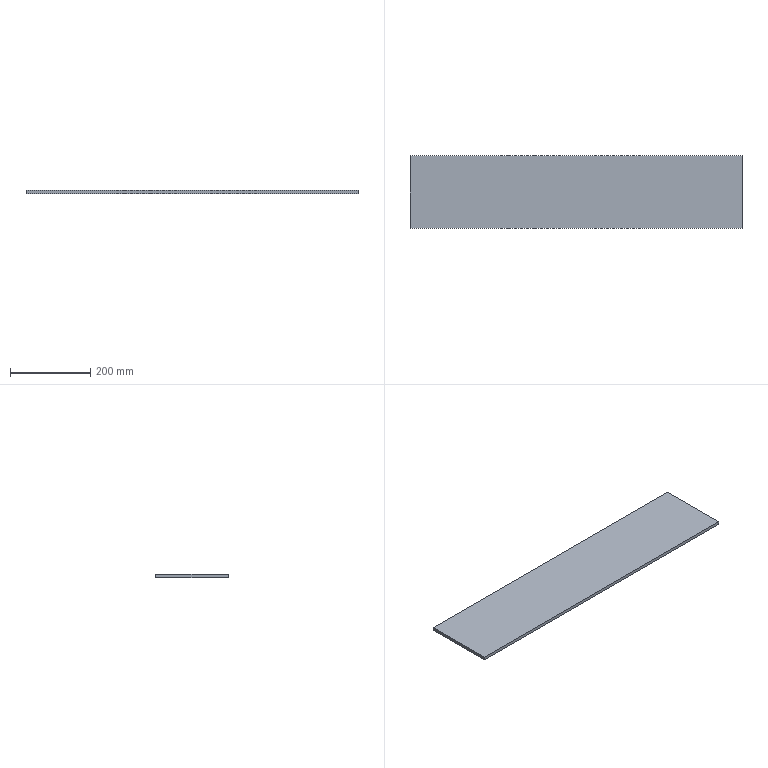Part | STEP file | 05-Steel plate 825x180x8 | 1 solid | 6 faces | box 825 x 180 x 8 mm | volume 1188000 mm3 | plane 6
STEP:
#1=CARTESIAN_POINT('',(0.,0.,0.));
#2=DIRECTION('',(0.,0.,1.));
#3=DIRECTION('',(1.,0.,0.));
#4=AXIS2_PLACEMENT_3D('',#1,#2,#3);
#5=CARTESIAN_POINT('',(0.,0.,0.));
#6=VERTEX_POINT('',#5);
#7=CARTESIAN_POINT('',(0.,-180.,0.));
#8=VERTEX_POINT('',#7);
#9=CARTESIAN_POINT('',(0.,0.,0.));
#10=DIRECTION('',(0.,-1.,0.));
#11=VECTOR('',#10,1.);
#12=LINE('',#9,#11);
#13=CARTESIAN_POINT('',(0.,0.,8.));
#14=DIRECTION('',(1.,0.,0.));
#15=DIRECTION('',(0.,1.,0.));
#16=AXIS2_PLACEMENT_3D('',#13,#14,#15);
#17=PLANE('',#16);
#18=CARTESIAN_POINT('',(0.,-8.));
#19=DIRECTION('',(-1.,0.));
#20=VECTOR('',#19,1.);
#21=LINE('',#18,#20);
#22=(GEOMETRIC_REPRESENTATION_CONTEXT(2)PARAMETRIC_REPRESENTATION_CONTEXT()REPRESENTATION_CONTEXT('',''));
#23=DEFINITIONAL_REPRESENTATION('',(#21),#22);
#24=PCURVE('',#17,#23);
#25=CARTESIAN_POINT('',(0.,0.,0.));
#26=DIRECTION('',(0.,0.,1.));
#27=DIRECTION('',(1.,0.,0.));
#28=AXIS2_PLACEMENT_3D('',#25,#26,#27);
#29=PLANE('',#28);
#30=CARTESIAN_POINT('',(0.,0.));
#31=DIRECTION('',(0.,-1.));
#32=VECTOR('',#31,1.);
#33=LINE('',#30,#32);
#34=(GEOMETRIC_REPRESENTATION_CONTEXT(2)PARAMETRIC_REPRESENTATION_CONTEXT()REPRESENTATION_CONTEXT('',''));
#35=DEFINITIONAL_REPRESENTATION('',(#33),#34);
#36=PCURVE('',#29,#35);
#37=SURFACE_CURVE('',#12,(#24,#36),.PCURVE_S1.);
#38=EDGE_CURVE('',#6,#8,#37,.T.);
#39=ORIENTED_EDGE('',*,*,#38,.T.);
#40=CARTESIAN_POINT('',(0.,-180.,8.));
#41=VERTEX_POINT('',#40);
#42=CARTESIAN_POINT('',(0.,-180.,8.));
#43=DIRECTION('',(0.,0.,-1.));
#44=VECTOR('',#43,1.);
#45=LINE('',#42,#44);
#46=CARTESIAN_POINT('',(-180.,0.));
#47=DIRECTION('',(0.,-1.));
#48=VECTOR('',#47,1.);
#49=LINE('',#46,#48);
#50=(GEOMETRIC_REPRESENTATION_CONTEXT(2)PARAMETRIC_REPRESENTATION_CONTEXT()REPRESENTATION_CONTEXT('',''));
#51=DEFINITIONAL_REPRESENTATION('',(#49),#50);
#52=PCURVE('',#17,#51);
#53=CARTESIAN_POINT('',(0.,-180.,8.));
#54=DIRECTION('',(0.,1.,0.));
#55=DIRECTION('',(0.,0.,1.));
#56=AXIS2_PLACEMENT_3D('',#53,#54,#55);
#57=PLANE('',#56);
#58=CARTESIAN_POINT('',(0.,0.));
#59=DIRECTION('',(-1.,0.));
#60=VECTOR('',#59,1.);
#61=LINE('',#58,#60);
#62=(GEOMETRIC_REPRESENTATION_CONTEXT(2)PARAMETRIC_REPRESENTATION_CONTEXT()REPRESENTATION_CONTEXT('',''));
#63=DEFINITIONAL_REPRESENTATION('',(#61),#62);
#64=PCURVE('',#57,#63);
#65=SURFACE_CURVE('',#45,(#52,#64),.PCURVE_S1.);
#66=EDGE_CURVE('',#41,#8,#65,.T.);
#67=ORIENTED_EDGE('',*,*,#66,.F.);
#68=CARTESIAN_POINT('',(0.,0.,8.));
#69=VERTEX_POINT('',#68);
#70=CARTESIAN_POINT('',(0.,0.,8.));
#71=DIRECTION('',(0.,-1.,0.));
#72=VECTOR('',#71,1.);
#73=LINE('',#70,#72);
#74=CARTESIAN_POINT('',(0.,0.));
#75=DIRECTION('',(-1.,0.));
#76=VECTOR('',#75,1.);
#77=LINE('',#74,#76);
#78=(GEOMETRIC_REPRESENTATION_CONTEXT(2)PARAMETRIC_REPRESENTATION_CONTEXT()REPRESENTATION_CONTEXT('',''));
#79=DEFINITIONAL_REPRESENTATION('',(#77),#78);
#80=PCURVE('',#17,#79);
#81=CARTESIAN_POINT('',(0.,0.,8.));
#82=DIRECTION('',(0.,0.,1.));
#83=DIRECTION('',(1.,0.,0.));
#84=AXIS2_PLACEMENT_3D('',#81,#82,#83);
#85=PLANE('',#84);
#86=CARTESIAN_POINT('',(0.,0.));
#87=DIRECTION('',(0.,-1.));
#88=VECTOR('',#87,1.);
#89=LINE('',#86,#88);
#90=(GEOMETRIC_REPRESENTATION_CONTEXT(2)PARAMETRIC_REPRESENTATION_CONTEXT()REPRESENTATION_CONTEXT('',''));
#91=DEFINITIONAL_REPRESENTATION('',(#89),#90);
#92=PCURVE('',#85,#91);
#93=SURFACE_CURVE('',#73,(#80,#92),.PCURVE_S1.);
#94=EDGE_CURVE('',#69,#41,#93,.T.);
#95=ORIENTED_EDGE('',*,*,#94,.F.);
#96=CARTESIAN_POINT('',(0.,0.,8.));
#97=DIRECTION('',(0.,0.,-1.));
#98=VECTOR('',#97,1.);
#99=LINE('',#96,#98);
#100=CARTESIAN_POINT('',(0.,0.));
#101=DIRECTION('',(0.,-1.));
#102=VECTOR('',#101,1.);
#103=LINE('',#100,#102);
#104=(GEOMETRIC_REPRESENTATION_CONTEXT(2)PARAMETRIC_REPRESENTATION_CONTEXT()REPRESENTATION_CONTEXT('',''));
#105=DEFINITIONAL_REPRESENTATION('',(#103),#104);
#106=PCURVE('',#17,#105);
#107=CARTESIAN_POINT('',(0.,0.,8.));
#108=DIRECTION('',(0.,-1.,0.));
#109=DIRECTION('',(0.,0.,-1.));
#110=AXIS2_PLACEMENT_3D('',#107,#108,#109);
#111=PLANE('',#110);
#112=CARTESIAN_POINT('',(0.,0.));
#113=DIRECTION('',(1.,0.));
#114=VECTOR('',#113,1.);
#115=LINE('',#112,#114);
#116=(GEOMETRIC_REPRESENTATION_CONTEXT(2)PARAMETRIC_REPRESENTATION_CONTEXT()REPRESENTATION_CONTEXT('',''));
#117=DEFINITIONAL_REPRESENTATION('',(#115),#116);
#118=PCURVE('',#111,#117);
#119=SURFACE_CURVE('',#99,(#106,#118),.PCURVE_S1.);
#120=EDGE_CURVE('',#69,#6,#119,.T.);
#121=ORIENTED_EDGE('',*,*,#120,.T.);
#122=EDGE_LOOP('',(#39,#67,#95,#121));
#123=FACE_BOUND('',#122,.T.);
#124=ADVANCED_FACE('',(#123),#17,.F.);
#125=CARTESIAN_POINT('',(825.,-180.,0.));
#126=VERTEX_POINT('',#125);
#127=CARTESIAN_POINT('',(0.,-180.,0.));
#128=DIRECTION('',(1.,0.,0.));
#129=VECTOR('',#128,1.);
#130=LINE('',#127,#129);
#131=CARTESIAN_POINT('',(-8.,0.));
#132=DIRECTION('',(0.,1.));
#133=VECTOR('',#132,1.);
#134=LINE('',#131,#133);
#135=(GEOMETRIC_REPRESENTATION_CONTEXT(2)PARAMETRIC_REPRESENTATION_CONTEXT()REPRESENTATION_CONTEXT('',''));
#136=DEFINITIONAL_REPRESENTATION('',(#134),#135);
#137=PCURVE('',#57,#136);
#138=CARTESIAN_POINT('',(0.,-180.));
#139=DIRECTION('',(1.,0.));
#140=VECTOR('',#139,1.);
#141=LINE('',#138,#140);
#142=(GEOMETRIC_REPRESENTATION_CONTEXT(2)PARAMETRIC_REPRESENTATION_CONTEXT()REPRESENTATION_CONTEXT('',''));
#143=DEFINITIONAL_REPRESENTATION('',(#141),#142);
#144=PCURVE('',#29,#143);
#145=SURFACE_CURVE('',#130,(#137,#144),.PCURVE_S1.);
#146=EDGE_CURVE('',#8,#126,#145,.T.);
#147=ORIENTED_EDGE('',*,*,#146,.T.);
#148=CARTESIAN_POINT('',(825.,-180.,8.));
#149=VERTEX_POINT('',#148);
#150=CARTESIAN_POINT('',(825.,-180.,8.));
#151=DIRECTION('',(0.,0.,-1.));
#152=VECTOR('',#151,1.);
#153=LINE('',#150,#152);
#154=CARTESIAN_POINT('',(0.,825.));
#155=DIRECTION('',(-1.,0.));
#156=VECTOR('',#155,1.);
#157=LINE('',#154,#156);
#158=(GEOMETRIC_REPRESENTATION_CONTEXT(2)PARAMETRIC_REPRESENTATION_CONTEXT()REPRESENTATION_CONTEXT('',''));
#159=DEFINITIONAL_REPRESENTATION('',(#157),#158);
#160=PCURVE('',#57,#159);
#161=CARTESIAN_POINT('',(825.,0.,8.));
#162=DIRECTION('',(-1.,0.,0.));
#163=DIRECTION('',(0.,0.,1.));
#164=AXIS2_PLACEMENT_3D('',#161,#162,#163);
#165=PLANE('',#164);
#166=CARTESIAN_POINT('',(0.,-180.));
#167=DIRECTION('',(-1.,0.));
#168=VECTOR('',#167,1.);
#169=LINE('',#166,#168);
#170=(GEOMETRIC_REPRESENTATION_CONTEXT(2)PARAMETRIC_REPRESENTATION_CONTEXT()REPRESENTATION_CONTEXT('',''));
#171=DEFINITIONAL_REPRESENTATION('',(#169),#170);
#172=PCURVE('',#165,#171);
#173=SURFACE_CURVE('',#153,(#160,#172),.PCURVE_S1.);
#174=EDGE_CURVE('',#149,#126,#173,.T.);
#175=ORIENTED_EDGE('',*,*,#174,.F.);
#176=CARTESIAN_POINT('',(0.,-180.,8.));
#177=DIRECTION('',(1.,0.,0.));
#178=VECTOR('',#177,1.);
#179=LINE('',#176,#178);
#180=CARTESIAN_POINT('',(0.,0.));
#181=DIRECTION('',(0.,1.));
#182=VECTOR('',#181,1.);
#183=LINE('',#180,#182);
#184=(GEOMETRIC_REPRESENTATION_CONTEXT(2)PARAMETRIC_REPRESENTATION_CONTEXT()REPRESENTATION_CONTEXT('',''));
#185=DEFINITIONAL_REPRESENTATION('',(#183),#184);
#186=PCURVE('',#57,#185);
#187=CARTESIAN_POINT('',(0.,-180.));
#188=DIRECTION('',(1.,0.));
#189=VECTOR('',#188,1.);
#190=LINE('',#187,#189);
#191=(GEOMETRIC_REPRESENTATION_CONTEXT(2)PARAMETRIC_REPRESENTATION_CONTEXT()REPRESENTATION_CONTEXT('',''));
#192=DEFINITIONAL_REPRESENTATION('',(#190),#191);
#193=PCURVE('',#85,#192);
#194=SURFACE_CURVE('',#179,(#186,#193),.PCURVE_S1.);
#195=EDGE_CURVE('',#41,#149,#194,.T.);
#196=ORIENTED_EDGE('',*,*,#195,.F.);
#197=ORIENTED_EDGE('',*,*,#66,.T.);
#198=EDGE_LOOP('',(#147,#175,#196,#197));
#199=FACE_BOUND('',#198,.T.);
#200=ADVANCED_FACE('',(#199),#57,.F.);
#201=CARTESIAN_POINT('',(825.,0.,0.));
#202=VERTEX_POINT('',#201);
#203=CARTESIAN_POINT('',(825.,0.,0.));
#204=DIRECTION('',(0.,1.,0.));
#205=VECTOR('',#204,1.);
#206=LINE('',#203,#205);
#207=CARTESIAN_POINT('',(-8.,0.));
#208=DIRECTION('',(0.,1.));
#209=VECTOR('',#208,1.);
#210=LINE('',#207,#209);
#211=(GEOMETRIC_REPRESENTATION_CONTEXT(2)PARAMETRIC_REPRESENTATION_CONTEXT()REPRESENTATION_CONTEXT('',''));
#212=DEFINITIONAL_REPRESENTATION('',(#210),#211);
#213=PCURVE('',#165,#212);
#214=CARTESIAN_POINT('',(825.,0.));
#215=DIRECTION('',(0.,1.));
#216=VECTOR('',#215,1.);
#217=LINE('',#214,#216);
#218=(GEOMETRIC_REPRESENTATION_CONTEXT(2)PARAMETRIC_REPRESENTATION_CONTEXT()REPRESENTATION_CONTEXT('',''));
#219=DEFINITIONAL_REPRESENTATION('',(#217),#218);
#220=PCURVE('',#29,#219);
#221=SURFACE_CURVE('',#206,(#213,#220),.PCURVE_S1.);
#222=EDGE_CURVE('',#126,#202,#221,.T.);
#223=ORIENTED_EDGE('',*,*,#222,.T.);
#224=CARTESIAN_POINT('',(825.,0.,8.));
#225=VERTEX_POINT('',#224);
#226=CARTESIAN_POINT('',(825.,0.,8.));
#227=DIRECTION('',(0.,0.,-1.));
#228=VECTOR('',#227,1.);
#229=LINE('',#226,#228);
#230=CARTESIAN_POINT('',(0.,0.));
#231=DIRECTION('',(-1.,0.));
#232=VECTOR('',#231,1.);
#233=LINE('',#230,#232);
#234=(GEOMETRIC_REPRESENTATION_CONTEXT(2)PARAMETRIC_REPRESENTATION_CONTEXT()REPRESENTATION_CONTEXT('',''));
#235=DEFINITIONAL_REPRESENTATION('',(#233),#234);
#236=PCURVE('',#165,#235);
#237=CARTESIAN_POINT('',(0.,825.));
#238=DIRECTION('',(1.,0.));
#239=VECTOR('',#238,1.);
#240=LINE('',#237,#239);
#241=(GEOMETRIC_REPRESENTATION_CONTEXT(2)PARAMETRIC_REPRESENTATION_CONTEXT()REPRESENTATION_CONTEXT('',''));
#242=DEFINITIONAL_REPRESENTATION('',(#240),#241);
#243=PCURVE('',#111,#242);
#244=SURFACE_CURVE('',#229,(#236,#243),.PCURVE_S1.);
#245=EDGE_CURVE('',#225,#202,#244,.T.);
#246=ORIENTED_EDGE('',*,*,#245,.F.);
#247=CARTESIAN_POINT('',(825.,0.,8.));
#248=DIRECTION('',(0.,1.,0.));
#249=VECTOR('',#248,1.);
#250=LINE('',#247,#249);
#251=CARTESIAN_POINT('',(0.,0.));
#252=DIRECTION('',(0.,1.));
#253=VECTOR('',#252,1.);
#254=LINE('',#251,#253);
#255=(GEOMETRIC_REPRESENTATION_CONTEXT(2)PARAMETRIC_REPRESENTATION_CONTEXT()REPRESENTATION_CONTEXT('',''));
#256=DEFINITIONAL_REPRESENTATION('',(#254),#255);
#257=PCURVE('',#165,#256);
#258=CARTESIAN_POINT('',(825.,0.));
#259=DIRECTION('',(0.,1.));
#260=VECTOR('',#259,1.);
#261=LINE('',#258,#260);
#262=(GEOMETRIC_REPRESENTATION_CONTEXT(2)PARAMETRIC_REPRESENTATION_CONTEXT()REPRESENTATION_CONTEXT('',''));
#263=DEFINITIONAL_REPRESENTATION('',(#261),#262);
#264=PCURVE('',#85,#263);
#265=SURFACE_CURVE('',#250,(#257,#264),.PCURVE_S1.);
#266=EDGE_CURVE('',#149,#225,#265,.T.);
#267=ORIENTED_EDGE('',*,*,#266,.F.);
#268=ORIENTED_EDGE('',*,*,#174,.T.);
#269=EDGE_LOOP('',(#223,#246,#267,#268));
#270=FACE_BOUND('',#269,.T.);
#271=ADVANCED_FACE('',(#270),#165,.F.);
#272=CARTESIAN_POINT('',(0.,0.,0.));
#273=DIRECTION('',(-1.,0.,0.));
#274=VECTOR('',#273,1.);
#275=LINE('',#272,#274);
#276=CARTESIAN_POINT('',(8.,0.));
#277=DIRECTION('',(0.,-1.));
#278=VECTOR('',#277,1.);
#279=LINE('',#276,#278);
#280=(GEOMETRIC_REPRESENTATION_CONTEXT(2)PARAMETRIC_REPRESENTATION_CONTEXT()REPRESENTATION_CONTEXT('',''));
#281=DEFINITIONAL_REPRESENTATION('',(#279),#280);
#282=PCURVE('',#111,#281);
#283=CARTESIAN_POINT('',(0.,0.));
#284=DIRECTION('',(-1.,0.));
#285=VECTOR('',#284,1.);
#286=LINE('',#283,#285);
#287=(GEOMETRIC_REPRESENTATION_CONTEXT(2)PARAMETRIC_REPRESENTATION_CONTEXT()REPRESENTATION_CONTEXT('',''));
#288=DEFINITIONAL_REPRESENTATION('',(#286),#287);
#289=PCURVE('',#29,#288);
#290=SURFACE_CURVE('',#275,(#282,#289),.PCURVE_S1.);
#291=EDGE_CURVE('',#202,#6,#290,.T.);
#292=ORIENTED_EDGE('',*,*,#291,.T.);
#293=ORIENTED_EDGE('',*,*,#120,.F.);
#294=CARTESIAN_POINT('',(0.,0.,8.));
#295=DIRECTION('',(-1.,0.,0.));
#296=VECTOR('',#295,1.);
#297=LINE('',#294,#296);
#298=CARTESIAN_POINT('',(0.,0.));
#299=DIRECTION('',(0.,-1.));
#300=VECTOR('',#299,1.);
#301=LINE('',#298,#300);
#302=(GEOMETRIC_REPRESENTATION_CONTEXT(2)PARAMETRIC_REPRESENTATION_CONTEXT()REPRESENTATION_CONTEXT('',''));
#303=DEFINITIONAL_REPRESENTATION('',(#301),#302);
#304=PCURVE('',#111,#303);
#305=CARTESIAN_POINT('',(0.,0.));
#306=DIRECTION('',(-1.,0.));
#307=VECTOR('',#306,1.);
#308=LINE('',#305,#307);
#309=(GEOMETRIC_REPRESENTATION_CONTEXT(2)PARAMETRIC_REPRESENTATION_CONTEXT()REPRESENTATION_CONTEXT('',''));
#310=DEFINITIONAL_REPRESENTATION('',(#308),#309);
#311=PCURVE('',#85,#310);
#312=SURFACE_CURVE('',#297,(#304,#311),.PCURVE_S1.);
#313=EDGE_CURVE('',#225,#69,#312,.T.);
#314=ORIENTED_EDGE('',*,*,#313,.F.);
#315=ORIENTED_EDGE('',*,*,#245,.T.);
#316=EDGE_LOOP('',(#292,#293,#314,#315));
#317=FACE_BOUND('',#316,.T.);
#318=ADVANCED_FACE('',(#317),#111,.F.);
#319=ORIENTED_EDGE('',*,*,#94,.T.);
#320=ORIENTED_EDGE('',*,*,#195,.T.);
#321=ORIENTED_EDGE('',*,*,#266,.T.);
#322=ORIENTED_EDGE('',*,*,#313,.T.);
#323=EDGE_LOOP('',(#319,#320,#321,#322));
#324=FACE_BOUND('',#323,.T.);
#325=ADVANCED_FACE('',(#324),#85,.T.);
#326=ORIENTED_EDGE('',*,*,#38,.F.);
#327=ORIENTED_EDGE('',*,*,#291,.F.);
#328=ORIENTED_EDGE('',*,*,#222,.F.);
#329=ORIENTED_EDGE('',*,*,#146,.F.);
#330=EDGE_LOOP('',(#326,#327,#328,#329));
#331=FACE_BOUND('',#330,.T.);
#332=ADVANCED_FACE('',(#331),#29,.F.);
#333=CLOSED_SHELL('',(#124,#200,#271,#318,#325,#332));
#334=MANIFOLD_SOLID_BREP('',#333);
#335=(LENGTH_UNIT()NAMED_UNIT(*)SI_UNIT(.MILLI.,.METRE.));
#336=UNCERTAINTY_MEASURE_WITH_UNIT(LENGTH_MEASURE(0.0000001),#335,'','');
#337=(NAMED_UNIT(*)PLANE_ANGLE_UNIT()SI_UNIT($,.RADIAN.));
#338=(NAMED_UNIT(*)SI_UNIT($,.STERADIAN.)SOLID_ANGLE_UNIT());
#339=(GEOMETRIC_REPRESENTATION_CONTEXT(3)GLOBAL_UNCERTAINTY_ASSIGNED_CONTEXT((#336))GLOBAL_UNIT_ASSIGNED_CONTEXT((#335,#337,#338))REPRESENTATION_CONTEXT('',''));
#340=ADVANCED_BREP_SHAPE_REPRESENTATION('',(#4,#334),#339);